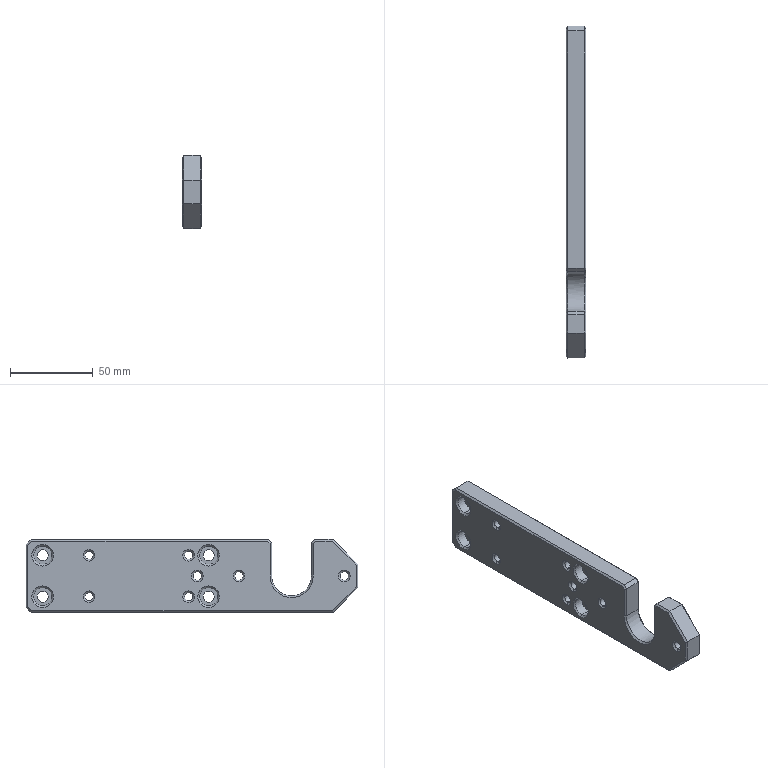Part | SolidWorks | features BaseBody 1 | 1 solid | 123 faces | box 12 x 200 x 44 mm | volume 88082 mm3 | cone 47 | plane 45 | cylinder 31 | commonest cylinder face diameters 5 x14 6.6 x8 11 x8 24 x1